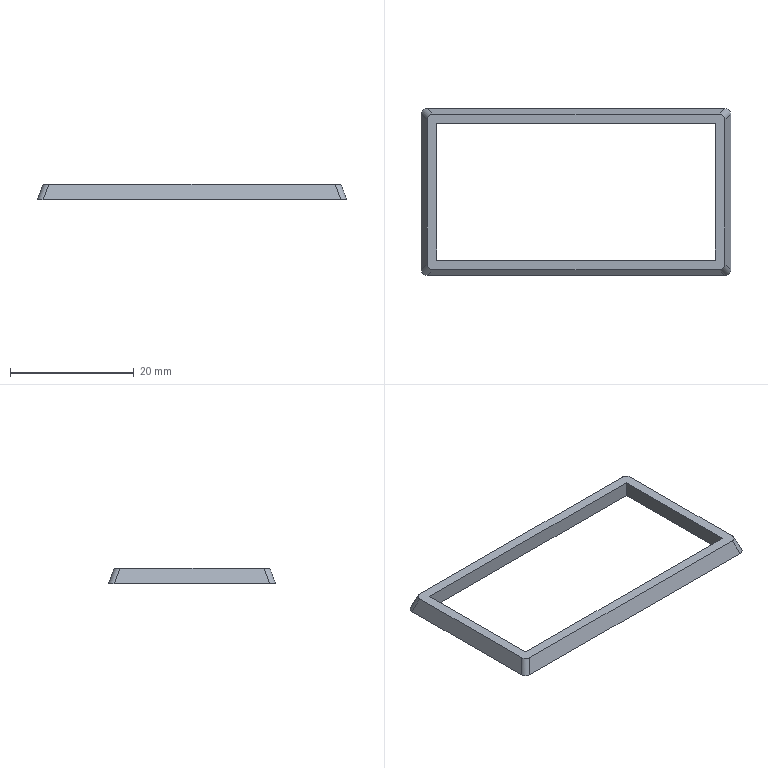Part | STEP file | Karet | 1 solid | 14 faces | box 50 x 27 x 2.5 mm | volume 725.773 mm3 | plane 10 | cylinder 4 | commonest cylinder face diameters 2 x4
STEP:
#1=CARTESIAN_POINT('',(0.,0.,0.));
#2=DIRECTION('',(0.,0.,1.));
#3=DIRECTION('',(1.,0.,0.));
#4=AXIS2_PLACEMENT_3D('',#1,#2,#3);
#5=CARTESIAN_POINT('',(24.09,-11.65,1.25));
#6=VERTEX_POINT('',#5);
#7=CARTESIAN_POINT('',(24.09,11.65,1.25));
#8=VERTEX_POINT('',#7);
#9=CARTESIAN_POINT('',(24.09,13.5,1.25));
#10=DIRECTION('',(0.,1.,0.));
#11=VECTOR('',#10,1.);
#12=LINE('',#9,#11);
#13=CARTESIAN_POINT('',(-25.,-13.5,1.25));
#14=DIRECTION('',(0.,0.,1.));
#15=DIRECTION('',(1.,0.,0.));
#16=AXIS2_PLACEMENT_3D('',#13,#14,#15);
#17=PLANE('',#16);
#18=CARTESIAN_POINT('',(49.09,27.));
#19=DIRECTION('',(0.,1.));
#20=VECTOR('',#19,1.);
#21=LINE('',#18,#20);
#22=(GEOMETRIC_REPRESENTATION_CONTEXT(2)PARAMETRIC_REPRESENTATION_CONTEXT()REPRESENTATION_CONTEXT('',''));
#23=DEFINITIONAL_REPRESENTATION('',(#21),#22);
#24=PCURVE('',#17,#23);
#25=CARTESIAN_POINT('',(24.09,-13.5,1.25));
#26=DIRECTION('',(0.9397,0.,0.342));
#27=DIRECTION('',(0.342,0.,-0.9397));
#28=AXIS2_PLACEMENT_3D('',#25,#26,#27);
#29=PLANE('',#28);
#30=CARTESIAN_POINT('',(0.,27.));
#31=DIRECTION('',(0.,1.));
#32=VECTOR('',#31,1.);
#33=LINE('',#30,#32);
#34=(GEOMETRIC_REPRESENTATION_CONTEXT(2)PARAMETRIC_REPRESENTATION_CONTEXT()REPRESENTATION_CONTEXT('',''));
#35=DEFINITIONAL_REPRESENTATION('',(#33),#34);
#36=PCURVE('',#29,#35);
#37=SURFACE_CURVE('',#12,(#24,#36),.PCURVE_S1.);
#38=EDGE_CURVE('',#6,#8,#37,.T.);
#39=ORIENTED_EDGE('',*,*,#38,.T.);
#40=CARTESIAN_POINT('',(23.15,12.59,1.25));
#41=VERTEX_POINT('',#40);
#42=CARTESIAN_POINT('',(24.09,11.65,1.25));
#43=CARTESIAN_POINT('',(24.09,12.213,1.25));
#44=CARTESIAN_POINT('',(23.713,12.59,1.25));
#45=CARTESIAN_POINT('',(23.15,12.59,1.25));
#46=(BOUNDED_CURVE()B_SPLINE_CURVE(3,(#42,#43,#44,#45),.UNSPECIFIED.,.F.,.F.)B_SPLINE_CURVE_WITH_KNOTS((4,4),(5.556,7.01),.PIECEWISE_BEZIER_KNOTS.)CURVE()GEOMETRIC_REPRESENTATION_ITEM()RATIONAL_B_SPLINE_CURVE((1.,0.8315,0.8315,1.))REPRESENTATION_ITEM(''));
#47=CARTESIAN_POINT('',(49.09,25.15));
#48=CARTESIAN_POINT('',(49.09,25.713));
#49=CARTESIAN_POINT('',(48.713,26.09));
#50=CARTESIAN_POINT('',(48.15,26.09));
#51=(BOUNDED_CURVE()B_SPLINE_CURVE(3,(#47,#48,#49,#50),.UNSPECIFIED.,.F.,.F.)B_SPLINE_CURVE_WITH_KNOTS((4,4),(5.556,7.01),.PIECEWISE_BEZIER_KNOTS.)CURVE()GEOMETRIC_REPRESENTATION_ITEM()RATIONAL_B_SPLINE_CURVE((1.,0.8315,0.8315,1.))REPRESENTATION_ITEM(''));
#52=(GEOMETRIC_REPRESENTATION_CONTEXT(2)PARAMETRIC_REPRESENTATION_CONTEXT()REPRESENTATION_CONTEXT('',''));
#53=DEFINITIONAL_REPRESENTATION('',(#51),#52);
#54=PCURVE('',#17,#53);
#55=CARTESIAN_POINT('',(18.108,6.608,14.763));
#56=DIRECTION('',(0.3236,0.3236,-0.8891));
#57=DIRECTION('',(-0.9397,0.,-0.342));
#58=AXIS2_PLACEMENT_3D('',#55,#56,#57);
#59=CYLINDRICAL_SURFACE('',#58,1.);
#60=CARTESIAN_POINT('',(3.142,15.582));
#61=CARTESIAN_POINT('',(3.121,15.589));
#62=CARTESIAN_POINT('',(3.081,15.603));
#63=CARTESIAN_POINT('',(3.018,15.622));
#64=CARTESIAN_POINT('',(2.955,15.639));
#65=CARTESIAN_POINT('',(2.89,15.656));
#66=CARTESIAN_POINT('',(2.824,15.67));
#67=CARTESIAN_POINT('',(2.757,15.683));
#68=CARTESIAN_POINT('',(2.69,15.693));
#69=CARTESIAN_POINT('',(2.622,15.702));
#70=CARTESIAN_POINT('',(2.553,15.708));
#71=CARTESIAN_POINT('',(2.484,15.711));
#72=CARTESIAN_POINT('',(2.415,15.713));
#73=CARTESIAN_POINT('',(2.346,15.711));
#74=CARTESIAN_POINT('',(2.277,15.708));
#75=CARTESIAN_POINT('',(2.208,15.702));
#76=CARTESIAN_POINT('',(2.14,15.693));
#77=CARTESIAN_POINT('',(2.072,15.683));
#78=CARTESIAN_POINT('',(2.006,15.67));
#79=CARTESIAN_POINT('',(1.94,15.656));
#80=CARTESIAN_POINT('',(1.875,15.639));
#81=CARTESIAN_POINT('',(1.811,15.622));
#82=CARTESIAN_POINT('',(1.749,15.603));
#83=CARTESIAN_POINT('',(1.708,15.589));
#84=CARTESIAN_POINT('',(1.688,15.582));
#85=B_SPLINE_CURVE_WITH_KNOTS('',3,(#60,#61,#62,#63,#64,#65,#66,#67,#68,#69,#70,#71,#72,#73,#74,#75,#76,#77,#78,#79,#80,#81,#82,#83,#84),.UNSPECIFIED.,.F.,.F.,(4,1,1,1,1,1,1,1,1,1,1,1,1,1,1,1,1,1,1,1,1,1,4),(5.556,5.622,5.689,5.755,5.821,5.887,5.953,6.019,6.085,6.151,6.217,6.283,6.349,6.415,6.481,6.547,6.614,6.68,6.746,6.812,6.878,6.944,7.01),.QUASI_UNIFORM_KNOTS.);
#86=(GEOMETRIC_REPRESENTATION_CONTEXT(2)PARAMETRIC_REPRESENTATION_CONTEXT()REPRESENTATION_CONTEXT('',''));
#87=DEFINITIONAL_REPRESENTATION('',(#85),#86);
#88=PCURVE('',#59,#87);
#89=SURFACE_CURVE('',#46,(#54,#88),.PCURVE_S1.);
#90=EDGE_CURVE('',#8,#41,#89,.T.);
#91=ORIENTED_EDGE('',*,*,#90,.T.);
#92=CARTESIAN_POINT('',(-23.15,12.59,1.25));
#93=VERTEX_POINT('',#92);
#94=CARTESIAN_POINT('',(-25.,12.59,1.25));
#95=DIRECTION('',(-1.,0.,0.));
#96=VECTOR('',#95,1.);
#97=LINE('',#94,#96);
#98=CARTESIAN_POINT('',(0.,26.09));
#99=DIRECTION('',(-1.,0.));
#100=VECTOR('',#99,1.);
#101=LINE('',#98,#100);
#102=(GEOMETRIC_REPRESENTATION_CONTEXT(2)PARAMETRIC_REPRESENTATION_CONTEXT()REPRESENTATION_CONTEXT('',''));
#103=DEFINITIONAL_REPRESENTATION('',(#101),#102);
#104=PCURVE('',#17,#103);
#105=CARTESIAN_POINT('',(-25.,12.59,1.25));
#106=DIRECTION('',(0.,0.9397,0.342));
#107=DIRECTION('',(0.,-0.342,0.9397));
#108=AXIS2_PLACEMENT_3D('',#105,#106,#107);
#109=PLANE('',#108);
#110=CARTESIAN_POINT('',(0.,0.));
#111=DIRECTION('',(0.,-1.));
#112=VECTOR('',#111,1.);
#113=LINE('',#110,#112);
#114=(GEOMETRIC_REPRESENTATION_CONTEXT(2)PARAMETRIC_REPRESENTATION_CONTEXT()REPRESENTATION_CONTEXT('',''));
#115=DEFINITIONAL_REPRESENTATION('',(#113),#114);
#116=PCURVE('',#109,#115);
#117=SURFACE_CURVE('',#97,(#104,#116),.PCURVE_S1.);
#118=EDGE_CURVE('',#41,#93,#117,.T.);
#119=ORIENTED_EDGE('',*,*,#118,.T.);
#120=CARTESIAN_POINT('',(-24.09,11.65,1.25));
#121=VERTEX_POINT('',#120);
#122=CARTESIAN_POINT('',(-23.15,12.59,1.25));
#123=CARTESIAN_POINT('',(-23.713,12.59,1.25));
#124=CARTESIAN_POINT('',(-24.09,12.213,1.25));
#125=CARTESIAN_POINT('',(-24.09,11.65,1.25));
#126=(BOUNDED_CURVE()B_SPLINE_CURVE(3,(#122,#123,#124,#125),.UNSPECIFIED.,.F.,.F.)B_SPLINE_CURVE_WITH_KNOTS((4,4),(5.556,7.01),.PIECEWISE_BEZIER_KNOTS.)CURVE()GEOMETRIC_REPRESENTATION_ITEM()RATIONAL_B_SPLINE_CURVE((1.,0.8315,0.8315,1.))REPRESENTATION_ITEM(''));
#127=CARTESIAN_POINT('',(1.85,26.09));
#128=CARTESIAN_POINT('',(1.287,26.09));
#129=CARTESIAN_POINT('',(0.9099,25.713));
#130=CARTESIAN_POINT('',(0.9099,25.15));
#131=(BOUNDED_CURVE()B_SPLINE_CURVE(3,(#127,#128,#129,#130),.UNSPECIFIED.,.F.,.F.)B_SPLINE_CURVE_WITH_KNOTS((4,4),(5.556,7.01),.PIECEWISE_BEZIER_KNOTS.)CURVE()GEOMETRIC_REPRESENTATION_ITEM()RATIONAL_B_SPLINE_CURVE((1.,0.8315,0.8315,1.))REPRESENTATION_ITEM(''));
#132=(GEOMETRIC_REPRESENTATION_CONTEXT(2)PARAMETRIC_REPRESENTATION_CONTEXT()REPRESENTATION_CONTEXT('',''));
#133=DEFINITIONAL_REPRESENTATION('',(#131),#132);
#134=PCURVE('',#17,#133);
#135=CARTESIAN_POINT('',(-20.516,9.016,8.145));
#136=DIRECTION('',(-0.3236,0.3236,-0.8891));
#137=DIRECTION('',(-0.9397,0.,0.342));
#138=AXIS2_PLACEMENT_3D('',#135,#136,#137);
#139=CYLINDRICAL_SURFACE('',#138,1.);
#140=CARTESIAN_POINT('',(1.454,8.139));
#141=CARTESIAN_POINT('',(1.433,8.146));
#142=CARTESIAN_POINT('',(1.393,8.159));
#143=CARTESIAN_POINT('',(1.33,8.178));
#144=CARTESIAN_POINT('',(1.267,8.196));
#145=CARTESIAN_POINT('',(1.202,8.212));
#146=CARTESIAN_POINT('',(1.136,8.227));
#147=CARTESIAN_POINT('',(1.069,8.24));
#148=CARTESIAN_POINT('',(1.002,8.25));
#149=CARTESIAN_POINT('',(0.9335,8.259));
#150=CARTESIAN_POINT('',(0.8649,8.265));
#151=CARTESIAN_POINT('',(0.7959,8.268));
#152=CARTESIAN_POINT('',(0.7268,8.27));
#153=CARTESIAN_POINT('',(0.6576,8.268));
#154=CARTESIAN_POINT('',(0.5887,8.265));
#155=CARTESIAN_POINT('',(0.52,8.259));
#156=CARTESIAN_POINT('',(0.4518,8.25));
#157=CARTESIAN_POINT('',(0.3843,8.24));
#158=CARTESIAN_POINT('',(0.3176,8.227));
#159=CARTESIAN_POINT('',(0.2517,8.212));
#160=CARTESIAN_POINT('',(0.1869,8.196));
#161=CARTESIAN_POINT('',(0.1233,8.178));
#162=CARTESIAN_POINT('',(0.06087,8.159));
#163=CARTESIAN_POINT('',(0.02013,8.146));
#164=CARTESIAN_POINT('',(0.,8.139));
#165=B_SPLINE_CURVE_WITH_KNOTS('',3,(#140,#141,#142,#143,#144,#145,#146,#147,#148,#149,#150,#151,#152,#153,#154,#155,#156,#157,#158,#159,#160,#161,#162,#163,#164),.UNSPECIFIED.,.F.,.F.,(4,1,1,1,1,1,1,1,1,1,1,1,1,1,1,1,1,1,1,1,1,1,4),(5.556,5.622,5.689,5.755,5.821,5.887,5.953,6.019,6.085,6.151,6.217,6.283,6.349,6.415,6.481,6.547,6.614,6.68,6.746,6.812,6.878,6.944,7.01),.QUASI_UNIFORM_KNOTS.);
#166=(GEOMETRIC_REPRESENTATION_CONTEXT(2)PARAMETRIC_REPRESENTATION_CONTEXT()REPRESENTATION_CONTEXT('',''));
#167=DEFINITIONAL_REPRESENTATION('',(#165),#166);
#168=PCURVE('',#139,#167);
#169=SURFACE_CURVE('',#126,(#134,#168),.PCURVE_S1.);
#170=EDGE_CURVE('',#93,#121,#169,.T.);
#171=ORIENTED_EDGE('',*,*,#170,.T.);
#172=CARTESIAN_POINT('',(-24.09,-11.65,1.25));
#173=VERTEX_POINT('',#172);
#174=CARTESIAN_POINT('',(-24.09,-13.5,1.25));
#175=DIRECTION('',(0.,-1.,0.));
#176=VECTOR('',#175,1.);
#177=LINE('',#174,#176);
#178=CARTESIAN_POINT('',(0.9099,0.));
#179=DIRECTION('',(0.,-1.));
#180=VECTOR('',#179,1.);
#181=LINE('',#178,#180);
#182=(GEOMETRIC_REPRESENTATION_CONTEXT(2)PARAMETRIC_REPRESENTATION_CONTEXT()REPRESENTATION_CONTEXT('',''));
#183=DEFINITIONAL_REPRESENTATION('',(#181),#182);
#184=PCURVE('',#17,#183);
#185=CARTESIAN_POINT('',(-24.09,-13.5,1.25));
#186=DIRECTION('',(-0.9397,0.,0.342));
#187=DIRECTION('',(0.342,0.,0.9397));
#188=AXIS2_PLACEMENT_3D('',#185,#186,#187);
#189=PLANE('',#188);
#190=CARTESIAN_POINT('',(0.,0.));
#191=DIRECTION('',(0.,-1.));
#192=VECTOR('',#191,1.);
#193=LINE('',#190,#192);
#194=(GEOMETRIC_REPRESENTATION_CONTEXT(2)PARAMETRIC_REPRESENTATION_CONTEXT()REPRESENTATION_CONTEXT('',''));
#195=DEFINITIONAL_REPRESENTATION('',(#193),#194);
#196=PCURVE('',#189,#195);
#197=SURFACE_CURVE('',#177,(#184,#196),.PCURVE_S1.);
#198=EDGE_CURVE('',#121,#173,#197,.T.);
#199=ORIENTED_EDGE('',*,*,#198,.T.);
#200=CARTESIAN_POINT('',(-23.15,-12.59,1.25));
#201=VERTEX_POINT('',#200);
#202=CARTESIAN_POINT('',(-24.09,-11.65,1.25));
#203=CARTESIAN_POINT('',(-24.09,-12.213,1.25));
#204=CARTESIAN_POINT('',(-23.713,-12.59,1.25));
#205=CARTESIAN_POINT('',(-23.15,-12.59,1.25));
#206=(BOUNDED_CURVE()B_SPLINE_CURVE(3,(#202,#203,#204,#205),.UNSPECIFIED.,.F.,.F.)B_SPLINE_CURVE_WITH_KNOTS((4,4),(2.415,3.868),.PIECEWISE_BEZIER_KNOTS.)CURVE()GEOMETRIC_REPRESENTATION_ITEM()RATIONAL_B_SPLINE_CURVE((1.,0.8315,0.8315,1.))REPRESENTATION_ITEM(''));
#207=CARTESIAN_POINT('',(0.9099,1.85));
#208=CARTESIAN_POINT('',(0.9099,1.287));
#209=CARTESIAN_POINT('',(1.287,0.9099));
#210=CARTESIAN_POINT('',(1.85,0.9099));
#211=(BOUNDED_CURVE()B_SPLINE_CURVE(3,(#207,#208,#209,#210),.UNSPECIFIED.,.F.,.F.)B_SPLINE_CURVE_WITH_KNOTS((4,4),(2.415,3.868),.PIECEWISE_BEZIER_KNOTS.)CURVE()GEOMETRIC_REPRESENTATION_ITEM()RATIONAL_B_SPLINE_CURVE((1.,0.8315,0.8315,1.))REPRESENTATION_ITEM(''));
#212=(GEOMETRIC_REPRESENTATION_CONTEXT(2)PARAMETRIC_REPRESENTATION_CONTEXT()REPRESENTATION_CONTEXT('',''));
#213=DEFINITIONAL_REPRESENTATION('',(#211),#212);
#214=PCURVE('',#17,#213);
#215=CARTESIAN_POINT('',(-23.344,-11.844,0.3758));
#216=DIRECTION('',(0.3236,0.3236,0.8891));
#217=DIRECTION('',(0.9397,0.,-0.342));
#218=AXIS2_PLACEMENT_3D('',#215,#216,#217);
#219=CYLINDRICAL_SURFACE('',#218,1.);
#220=CARTESIAN_POINT('',(3.142,0.5986));
#221=CARTESIAN_POINT('',(3.162,0.5917));
#222=CARTESIAN_POINT('',(3.202,0.5782));
#223=CARTESIAN_POINT('',(3.265,0.5591));
#224=CARTESIAN_POINT('',(3.329,0.5414));
#225=CARTESIAN_POINT('',(3.393,0.5252));
#226=CARTESIAN_POINT('',(3.459,0.5107));
#227=CARTESIAN_POINT('',(3.526,0.498));
#228=CARTESIAN_POINT('',(3.593,0.4875));
#229=CARTESIAN_POINT('',(3.662,0.4791));
#230=CARTESIAN_POINT('',(3.73,0.473));
#231=CARTESIAN_POINT('',(3.799,0.4693));
#232=CARTESIAN_POINT('',(3.868,0.4681));
#233=CARTESIAN_POINT('',(3.938,0.4693));
#234=CARTESIAN_POINT('',(4.006,0.473));
#235=CARTESIAN_POINT('',(4.075,0.4791));
#236=CARTESIAN_POINT('',(4.143,0.4875));
#237=CARTESIAN_POINT('',(4.211,0.498));
#238=CARTESIAN_POINT('',(4.278,0.5107));
#239=CARTESIAN_POINT('',(4.343,0.5252));
#240=CARTESIAN_POINT('',(4.408,0.5414));
#241=CARTESIAN_POINT('',(4.472,0.5591));
#242=CARTESIAN_POINT('',(4.534,0.5782));
#243=CARTESIAN_POINT('',(4.575,0.5917));
#244=CARTESIAN_POINT('',(4.595,0.5986));
#245=B_SPLINE_CURVE_WITH_KNOTS('',3,(#220,#221,#222,#223,#224,#225,#226,#227,#228,#229,#230,#231,#232,#233,#234,#235,#236,#237,#238,#239,#240,#241,#242,#243,#244),.UNSPECIFIED.,.F.,.F.,(4,1,1,1,1,1,1,1,1,1,1,1,1,1,1,1,1,1,1,1,1,1,4),(2.415,2.481,2.547,2.613,2.679,2.745,2.811,2.877,2.943,3.009,3.076,3.142,3.208,3.274,3.34,3.406,3.472,3.538,3.604,3.67,3.736,3.802,3.868),.QUASI_UNIFORM_KNOTS.);
#246=(GEOMETRIC_REPRESENTATION_CONTEXT(2)PARAMETRIC_REPRESENTATION_CONTEXT()REPRESENTATION_CONTEXT('',''));
#247=DEFINITIONAL_REPRESENTATION('',(#245),#246);
#248=PCURVE('',#219,#247);
#249=SURFACE_CURVE('',#206,(#214,#248),.PCURVE_S1.);
#250=EDGE_CURVE('',#173,#201,#249,.T.);
#251=ORIENTED_EDGE('',*,*,#250,.T.);
#252=CARTESIAN_POINT('',(23.15,-12.59,1.25));
#253=VERTEX_POINT('',#252);
#254=CARTESIAN_POINT('',(25.,-12.59,1.25));
#255=DIRECTION('',(1.,0.,0.));
#256=VECTOR('',#255,1.);
#257=LINE('',#254,#256);
#258=CARTESIAN_POINT('',(50.,0.9099));
#259=DIRECTION('',(1.,0.));
#260=VECTOR('',#259,1.);
#261=LINE('',#258,#260);
#262=(GEOMETRIC_REPRESENTATION_CONTEXT(2)PARAMETRIC_REPRESENTATION_CONTEXT()REPRESENTATION_CONTEXT('',''));
#263=DEFINITIONAL_REPRESENTATION('',(#261),#262);
#264=PCURVE('',#17,#263);
#265=CARTESIAN_POINT('',(-25.,-12.59,1.25));
#266=DIRECTION('',(0.,-0.9397,0.342));
#267=DIRECTION('',(0.,-0.342,-0.9397));
#268=AXIS2_PLACEMENT_3D('',#265,#266,#267);
#269=PLANE('',#268);
#270=CARTESIAN_POINT('',(0.,50.));
#271=DIRECTION('',(0.,1.));
#272=VECTOR('',#271,1.);
#273=LINE('',#270,#272);
#274=(GEOMETRIC_REPRESENTATION_CONTEXT(2)PARAMETRIC_REPRESENTATION_CONTEXT()REPRESENTATION_CONTEXT('',''));
#275=DEFINITIONAL_REPRESENTATION('',(#273),#274);
#276=PCURVE('',#269,#275);
#277=SURFACE_CURVE('',#257,(#264,#276),.PCURVE_S1.);
#278=EDGE_CURVE('',#201,#253,#277,.T.);
#279=ORIENTED_EDGE('',*,*,#278,.T.);
#280=CARTESIAN_POINT('',(23.15,-12.59,1.25));
#281=CARTESIAN_POINT('',(23.713,-12.59,1.25));
#282=CARTESIAN_POINT('',(24.09,-12.213,1.25));
#283=CARTESIAN_POINT('',(24.09,-11.65,1.25));
#284=(BOUNDED_CURVE()B_SPLINE_CURVE(3,(#280,#281,#282,#283),.UNSPECIFIED.,.F.,.F.)B_SPLINE_CURVE_WITH_KNOTS((4,4),(2.415,3.868),.PIECEWISE_BEZIER_KNOTS.)CURVE()GEOMETRIC_REPRESENTATION_ITEM()RATIONAL_B_SPLINE_CURVE((1.,0.8315,0.8315,1.))REPRESENTATION_ITEM(''));
#285=CARTESIAN_POINT('',(48.15,0.9099));
#286=CARTESIAN_POINT('',(48.713,0.9099));
#287=CARTESIAN_POINT('',(49.09,1.287));
#288=CARTESIAN_POINT('',(49.09,1.85));
#289=(BOUNDED_CURVE()B_SPLINE_CURVE(3,(#285,#286,#287,#288),.UNSPECIFIED.,.F.,.F.)B_SPLINE_CURVE_WITH_KNOTS((4,4),(2.415,3.868),.PIECEWISE_BEZIER_KNOTS.)CURVE()GEOMETRIC_REPRESENTATION_ITEM()RATIONAL_B_SPLINE_CURVE((1.,0.8315,0.8315,1.))REPRESENTATION_ITEM(''));
#290=(GEOMETRIC_REPRESENTATION_CONTEXT(2)PARAMETRIC_REPRESENTATION_CONTEXT()REPRESENTATION_CONTEXT('',''));
#291=DEFINITIONAL_REPRESENTATION('',(#289),#290);
#292=PCURVE('',#17,#291);
#293=CARTESIAN_POINT('',(18.108,-6.608,14.763));
#294=DIRECTION('',(-0.3236,0.3236,0.8891));
#295=DIRECTION('',(0.9397,0.,0.342));
#296=AXIS2_PLACEMENT_3D('',#293,#294,#295);
#297=CYLINDRICAL_SURFACE('',#296,1.);
#298=CARTESIAN_POINT('',(4.83,-15.582));
#299=CARTESIAN_POINT('',(4.85,-15.589));
#300=CARTESIAN_POINT('',(4.891,-15.603));
#301=CARTESIAN_POINT('',(4.953,-15.622));
#302=CARTESIAN_POINT('',(5.017,-15.639));
#303=CARTESIAN_POINT('',(5.081,-15.656));
#304=CARTESIAN_POINT('',(5.147,-15.67));
#305=CARTESIAN_POINT('',(5.214,-15.683));
#306=CARTESIAN_POINT('',(5.281,-15.693));
#307=CARTESIAN_POINT('',(5.35,-15.702));
#308=CARTESIAN_POINT('',(5.418,-15.708));
#309=CARTESIAN_POINT('',(5.487,-15.711));
#310=CARTESIAN_POINT('',(5.556,-15.713));
#311=CARTESIAN_POINT('',(5.626,-15.711));
#312=CARTESIAN_POINT('',(5.695,-15.708));
#313=CARTESIAN_POINT('',(5.763,-15.702));
#314=CARTESIAN_POINT('',(5.831,-15.693));
#315=CARTESIAN_POINT('',(5.899,-15.683));
#316=CARTESIAN_POINT('',(5.966,-15.67));
#317=CARTESIAN_POINT('',(6.031,-15.656));
#318=CARTESIAN_POINT('',(6.096,-15.639));
#319=CARTESIAN_POINT('',(6.16,-15.622));
#320=CARTESIAN_POINT('',(6.222,-15.603));
#321=CARTESIAN_POINT('',(6.263,-15.589));
#322=CARTESIAN_POINT('',(6.283,-15.582));
#323=B_SPLINE_CURVE_WITH_KNOTS('',3,(#298,#299,#300,#301,#302,#303,#304,#305,#306,#307,#308,#309,#310,#311,#312,#313,#314,#315,#316,#317,#318,#319,#320,#321,#322),.UNSPECIFIED.,.F.,.F.,(4,1,1,1,1,1,1,1,1,1,1,1,1,1,1,1,1,1,1,1,1,1,4),(2.415,2.481,2.547,2.613,2.679,2.745,2.811,2.877,2.943,3.009,3.076,3.142,3.208,3.274,3.34,3.406,3.472,3.538,3.604,3.67,3.736,3.802,3.868),.QUASI_UNIFORM_KNOTS.);
#324=(GEOMETRIC_REPRESENTATION_CONTEXT(2)PARAMETRIC_REPRESENTATION_CONTEXT()REPRESENTATION_CONTEXT('',''));
#325=DEFINITIONAL_REPRESENTATION('',(#323),#324);
#326=PCURVE('',#297,#325);
#327=SURFACE_CURVE('',#284,(#292,#326),.PCURVE_S1.);
#328=EDGE_CURVE('',#253,#6,#327,.T.);
#329=ORIENTED_EDGE('',*,*,#328,.T.);
#330=EDGE_LOOP('',(#39,#91,#119,#171,#199,#251,#279,#329));
#331=FACE_BOUND('',#330,.T.);
#332=CARTESIAN_POINT('',(22.5,11.,1.25));
#333=VERTEX_POINT('',#332);
#334=CARTESIAN_POINT('',(-22.5,11.,1.25));
#335=VERTEX_POINT('',#334);
#336=CARTESIAN_POINT('',(-22.5,11.,1.25));
#337=DIRECTION('',(-1.,0.,0.));
#338=VECTOR('',#337,1.);
#339=LINE('',#336,#338);
#340=CARTESIAN_POINT('',(2.5,24.5));
#341=DIRECTION('',(-1.,0.));
#342=VECTOR('',#341,1.);
#343=LINE('',#340,#342);
#344=(GEOMETRIC_REPRESENTATION_CONTEXT(2)PARAMETRIC_REPRESENTATION_CONTEXT()REPRESENTATION_CONTEXT('',''));
#345=DEFINITIONAL_REPRESENTATION('',(#343),#344);
#346=PCURVE('',#17,#345);
#347=CARTESIAN_POINT('',(-22.5,11.,1.25));
#348=DIRECTION('',(0.,-1.,0.));
#349=DIRECTION('',(0.,0.,-1.));
#350=AXIS2_PLACEMENT_3D('',#347,#348,#349);
#351=PLANE('',#350);
#352=CARTESIAN_POINT('',(0.,0.));
#353=DIRECTION('',(0.,-1.));
#354=VECTOR('',#353,1.);
#355=LINE('',#352,#354);
#356=(GEOMETRIC_REPRESENTATION_CONTEXT(2)PARAMETRIC_REPRESENTATION_CONTEXT()REPRESENTATION_CONTEXT('',''));
#357=DEFINITIONAL_REPRESENTATION('',(#355),#356);
#358=PCURVE('',#351,#357);
#359=SURFACE_CURVE('',#339,(#346,#358),.PCURVE_S1.);
#360=EDGE_CURVE('',#333,#335,#359,.T.);
#361=ORIENTED_EDGE('',*,*,#360,.F.);
#362=CARTESIAN_POINT('',(22.5,-11.,1.25));
#363=VERTEX_POINT('',#362);
#364=CARTESIAN_POINT('',(22.5,11.,1.25));
#365=DIRECTION('',(0.,1.,0.));
#366=VECTOR('',#365,1.);
#367=LINE('',#364,#366);
#368=CARTESIAN_POINT('',(47.5,24.5));
#369=DIRECTION('',(0.,1.));
#370=VECTOR('',#369,1.);
#371=LINE('',#368,#370);
#372=(GEOMETRIC_REPRESENTATION_CONTEXT(2)PARAMETRIC_REPRESENTATION_CONTEXT()REPRESENTATION_CONTEXT('',''));
#373=DEFINITIONAL_REPRESENTATION('',(#371),#372);
#374=PCURVE('',#17,#373);
#375=CARTESIAN_POINT('',(22.5,11.,1.25));
#376=DIRECTION('',(-1.,0.,0.));
#377=DIRECTION('',(0.,-1.,0.));
#378=AXIS2_PLACEMENT_3D('',#375,#376,#377);
#379=PLANE('',#378);
#380=CARTESIAN_POINT('',(0.,0.));
#381=DIRECTION('',(-1.,0.));
#382=VECTOR('',#381,1.);
#383=LINE('',#380,#382);
#384=(GEOMETRIC_REPRESENTATION_CONTEXT(2)PARAMETRIC_REPRESENTATION_CONTEXT()REPRESENTATION_CONTEXT('',''));
#385=DEFINITIONAL_REPRESENTATION('',(#383),#384);
#386=PCURVE('',#379,#385);
#387=SURFACE_CURVE('',#367,(#374,#386),.PCURVE_S1.);
#388=EDGE_CURVE('',#363,#333,#387,.T.);
#389=ORIENTED_EDGE('',*,*,#388,.F.);
#390=CARTESIAN_POINT('',(-22.5,-11.,1.25));
#391=VERTEX_POINT('',#390);
#392=CARTESIAN_POINT('',(-22.5,-11.,1.25));
#393=DIRECTION('',(1.,0.,0.));
#394=VECTOR('',#393,1.);
#395=LINE('',#392,#394);
#396=CARTESIAN_POINT('',(2.5,2.5));
#397=DIRECTION('',(1.,0.));
#398=VECTOR('',#397,1.);
#399=LINE('',#396,#398);
#400=(GEOMETRIC_REPRESENTATION_CONTEXT(2)PARAMETRIC_REPRESENTATION_CONTEXT()REPRESENTATION_CONTEXT('',''));
#401=DEFINITIONAL_REPRESENTATION('',(#399),#400);
#402=PCURVE('',#17,#401);
#403=CARTESIAN_POINT('',(-22.5,-11.,1.25));
#404=DIRECTION('',(0.,1.,0.));
#405=DIRECTION('',(0.,0.,1.));
#406=AXIS2_PLACEMENT_3D('',#403,#404,#405);
#407=PLANE('',#406);
#408=CARTESIAN_POINT('',(0.,0.));
#409=DIRECTION('',(0.,1.));
#410=VECTOR('',#409,1.);
#411=LINE('',#408,#410);
#412=(GEOMETRIC_REPRESENTATION_CONTEXT(2)PARAMETRIC_REPRESENTATION_CONTEXT()REPRESENTATION_CONTEXT('',''));
#413=DEFINITIONAL_REPRESENTATION('',(#411),#412);
#414=PCURVE('',#407,#413);
#415=SURFACE_CURVE('',#395,(#402,#414),.PCURVE_S1.);
#416=EDGE_CURVE('',#391,#363,#415,.T.);
#417=ORIENTED_EDGE('',*,*,#416,.F.);
#418=CARTESIAN_POINT('',(-22.5,11.,1.25));
#419=DIRECTION('',(0.,-1.,0.));
#420=VECTOR('',#419,1.);
#421=LINE('',#418,#420);
#422=CARTESIAN_POINT('',(2.5,24.5));
#423=DIRECTION('',(0.,-1.));
#424=VECTOR('',#423,1.);
#425=LINE('',#422,#424);
#426=(GEOMETRIC_REPRESENTATION_CONTEXT(2)PARAMETRIC_REPRESENTATION_CONTEXT()REPRESENTATION_CONTEXT('',''));
#427=DEFINITIONAL_REPRESENTATION('',(#425),#426);
#428=PCURVE('',#17,#427);
#429=CARTESIAN_POINT('',(-22.5,11.,1.25));
#430=DIRECTION('',(1.,0.,0.));
#431=DIRECTION('',(0.,1.,0.));
#432=AXIS2_PLACEMENT_3D('',#429,#430,#431);
#433=PLANE('',#432);
#434=CARTESIAN_POINT('',(0.,0.));
#435=DIRECTION('',(-1.,0.));
#436=VECTOR('',#435,1.);
#437=LINE('',#434,#436);
#438=(GEOMETRIC_REPRESENTATION_CONTEXT(2)PARAMETRIC_REPRESENTATION_CONTEXT()REPRESENTATION_CONTEXT('',''));
#439=DEFINITIONAL_REPRESENTATION('',(#437),#438);
#440=PCURVE('',#433,#439);
#441=SURFACE_CURVE('',#421,(#428,#440),.PCURVE_S1.);
#442=EDGE_CURVE('',#335,#391,#441,.T.);
#443=ORIENTED_EDGE('',*,*,#442,.F.);
#444=EDGE_LOOP('',(#361,#389,#417,#443));
#445=FACE_BOUND('',#444,.T.);
#446=ADVANCED_FACE('',(#331,#445),#17,.T.);
#447=CARTESIAN_POINT('',(24.06,13.5,-1.25));
#448=VERTEX_POINT('',#447);
#449=CARTESIAN_POINT('',(-24.06,13.5,-1.25));
#450=VERTEX_POINT('',#449);
#451=CARTESIAN_POINT('',(-25.,13.5,-1.25));
#452=DIRECTION('',(-1.,0.,0.));
#453=VECTOR('',#452,1.);
#454=LINE('',#451,#453);
#455=CARTESIAN_POINT('',(-25.,-13.5,-1.25));
#456=DIRECTION('',(0.,0.,1.));
#457=DIRECTION('',(1.,0.,0.));
#458=AXIS2_PLACEMENT_3D('',#455,#456,#457);
#459=PLANE('',#458);
#460=CARTESIAN_POINT('',(0.,27.));
#461=DIRECTION('',(-1.,0.));
#462=VECTOR('',#461,1.);
#463=LINE('',#460,#462);
#464=(GEOMETRIC_REPRESENTATION_CONTEXT(2)PARAMETRIC_REPRESENTATION_CONTEXT()REPRESENTATION_CONTEXT('',''));
#465=DEFINITIONAL_REPRESENTATION('',(#463),#464);
#466=PCURVE('',#459,#465);
#467=CARTESIAN_POINT('',(-2.66,0.));
#468=DIRECTION('',(0.,-1.));
#469=VECTOR('',#468,1.);
#470=LINE('',#467,#469);
#471=(GEOMETRIC_REPRESENTATION_CONTEXT(2)PARAMETRIC_REPRESENTATION_CONTEXT()REPRESENTATION_CONTEXT('',''));
#472=DEFINITIONAL_REPRESENTATION('',(#470),#471);
#473=PCURVE('',#109,#472);
#474=SURFACE_CURVE('',#454,(#466,#473),.PCURVE_S1.);
#475=EDGE_CURVE('',#448,#450,#474,.T.);
#476=ORIENTED_EDGE('',*,*,#475,.F.);
#477=CARTESIAN_POINT('',(25.,12.56,-1.25));
#478=VERTEX_POINT('',#477);
#479=CARTESIAN_POINT('',(24.06,13.5,-1.25));
#480=CARTESIAN_POINT('',(24.623,13.5,-1.25));
#481=CARTESIAN_POINT('',(25.,13.123,-1.25));
#482=CARTESIAN_POINT('',(25.,12.56,-1.25));
#483=(BOUNDED_CURVE()B_SPLINE_CURVE(3,(#479,#480,#481,#482),.UNSPECIFIED.,.F.,.F.)B_SPLINE_CURVE_WITH_KNOTS((4,4),(5.556,7.01),.PIECEWISE_BEZIER_KNOTS.)CURVE()GEOMETRIC_REPRESENTATION_ITEM()RATIONAL_B_SPLINE_CURVE((1.,0.8315,0.8315,1.))REPRESENTATION_ITEM(''));
#484=CARTESIAN_POINT('',(49.06,27.));
#485=CARTESIAN_POINT('',(49.623,27.));
#486=CARTESIAN_POINT('',(50.,26.623));
#487=CARTESIAN_POINT('',(50.,26.06));
#488=(BOUNDED_CURVE()B_SPLINE_CURVE(3,(#484,#485,#486,#487),.UNSPECIFIED.,.F.,.F.)B_SPLINE_CURVE_WITH_KNOTS((4,4),(5.556,7.01),.PIECEWISE_BEZIER_KNOTS.)CURVE()GEOMETRIC_REPRESENTATION_ITEM()RATIONAL_B_SPLINE_CURVE((1.,0.8315,0.8315,1.))REPRESENTATION_ITEM(''));
#489=(GEOMETRIC_REPRESENTATION_CONTEXT(2)PARAMETRIC_REPRESENTATION_CONTEXT()REPRESENTATION_CONTEXT('',''));
#490=DEFINITIONAL_REPRESENTATION('',(#488),#489);
#491=PCURVE('',#459,#490);
#492=CARTESIAN_POINT('',(1.688,18.394));
#493=CARTESIAN_POINT('',(1.708,18.401));
#494=CARTESIAN_POINT('',(1.749,18.414));
#495=CARTESIAN_POINT('',(1.811,18.433));
#496=CARTESIAN_POINT('',(1.875,18.451));
#497=CARTESIAN_POINT('',(1.94,18.467));
#498=CARTESIAN_POINT('',(2.006,18.482));
#499=CARTESIAN_POINT('',(2.072,18.494));
#500=CARTESIAN_POINT('',(2.14,18.505));
#501=CARTESIAN_POINT('',(2.208,18.513));
#502=CARTESIAN_POINT('',(2.277,18.52));
#503=CARTESIAN_POINT('',(2.346,18.523));
#504=CARTESIAN_POINT('',(2.415,18.524));
#505=CARTESIAN_POINT('',(2.484,18.523));
#506=CARTESIAN_POINT('',(2.553,18.52));
#507=CARTESIAN_POINT('',(2.622,18.513));
#508=CARTESIAN_POINT('',(2.69,18.505));
#509=CARTESIAN_POINT('',(2.757,18.494));
#510=CARTESIAN_POINT('',(2.824,18.482));
#511=CARTESIAN_POINT('',(2.89,18.467));
#512=CARTESIAN_POINT('',(2.955,18.451));
#513=CARTESIAN_POINT('',(3.018,18.433));
#514=CARTESIAN_POINT('',(3.081,18.414));
#515=CARTESIAN_POINT('',(3.121,18.401));
#516=CARTESIAN_POINT('',(3.142,18.394));
#517=B_SPLINE_CURVE_WITH_KNOTS('',3,(#492,#493,#494,#495,#496,#497,#498,#499,#500,#501,#502,#503,#504,#505,#506,#507,#508,#509,#510,#511,#512,#513,#514,#515,#516),.UNSPECIFIED.,.F.,.F.,(4,1,1,1,1,1,1,1,1,1,1,1,1,1,1,1,1,1,1,1,1,1,4),(5.556,5.622,5.689,5.755,5.821,5.887,5.953,6.019,6.085,6.151,6.217,6.283,6.349,6.415,6.481,6.547,6.614,6.68,6.746,6.812,6.878,6.944,7.01),.QUASI_UNIFORM_KNOTS.);
#518=(GEOMETRIC_REPRESENTATION_CONTEXT(2)PARAMETRIC_REPRESENTATION_CONTEXT()REPRESENTATION_CONTEXT('',''));
#519=DEFINITIONAL_REPRESENTATION('',(#517),#518);
#520=PCURVE('',#59,#519);
#521=SURFACE_CURVE('',#483,(#491,#520),.PCURVE_S1.);
#522=EDGE_CURVE('',#448,#478,#521,.T.);
#523=ORIENTED_EDGE('',*,*,#522,.T.);
#524=CARTESIAN_POINT('',(25.,-12.56,-1.25));
#525=VERTEX_POINT('',#524);
#526=CARTESIAN_POINT('',(25.,13.5,-1.25));
#527=DIRECTION('',(0.,1.,0.));
#528=VECTOR('',#527,1.);
#529=LINE('',#526,#528);
#530=CARTESIAN_POINT('',(50.,27.));
#531=DIRECTION('',(0.,1.));
#532=VECTOR('',#531,1.);
#533=LINE('',#530,#532);
#534=(GEOMETRIC_REPRESENTATION_CONTEXT(2)PARAMETRIC_REPRESENTATION_CONTEXT()REPRESENTATION_CONTEXT('',''));
#535=DEFINITIONAL_REPRESENTATION('',(#533),#534);
#536=PCURVE('',#459,#535);
#537=CARTESIAN_POINT('',(2.66,27.));
#538=DIRECTION('',(0.,1.));
#539=VECTOR('',#538,1.);
#540=LINE('',#537,#539);
#541=(GEOMETRIC_REPRESENTATION_CONTEXT(2)PARAMETRIC_REPRESENTATION_CONTEXT()REPRESENTATION_CONTEXT('',''));
#542=DEFINITIONAL_REPRESENTATION('',(#540),#541);
#543=PCURVE('',#29,#542);
#544=SURFACE_CURVE('',#529,(#536,#543),.PCURVE_S1.);
#545=EDGE_CURVE('',#525,#478,#544,.T.);
#546=ORIENTED_EDGE('',*,*,#545,.F.);
#547=CARTESIAN_POINT('',(24.06,-13.5,-1.25));
#548=VERTEX_POINT('',#547);
#549=CARTESIAN_POINT('',(25.,-12.56,-1.25));
#550=CARTESIAN_POINT('',(25.,-13.123,-1.25));
#551=CARTESIAN_POINT('',(24.623,-13.5,-1.25));
#552=CARTESIAN_POINT('',(24.06,-13.5,-1.25));
#553=(BOUNDED_CURVE()B_SPLINE_CURVE(3,(#549,#550,#551,#552),.UNSPECIFIED.,.F.,.F.)B_SPLINE_CURVE_WITH_KNOTS((4,4),(2.415,3.868),.PIECEWISE_BEZIER_KNOTS.)CURVE()GEOMETRIC_REPRESENTATION_ITEM()RATIONAL_B_SPLINE_CURVE((1.,0.8315,0.8315,1.))REPRESENTATION_ITEM(''));
#554=CARTESIAN_POINT('',(50.,0.9397));
#555=CARTESIAN_POINT('',(50.,0.3767));
#556=CARTESIAN_POINT('',(49.623,0.));
#557=CARTESIAN_POINT('',(49.06,0.));
#558=(BOUNDED_CURVE()B_SPLINE_CURVE(3,(#554,#555,#556,#557),.UNSPECIFIED.,.F.,.F.)B_SPLINE_CURVE_WITH_KNOTS((4,4),(2.415,3.868),.PIECEWISE_BEZIER_KNOTS.)CURVE()GEOMETRIC_REPRESENTATION_ITEM()RATIONAL_B_SPLINE_CURVE((1.,0.8315,0.8315,1.))REPRESENTATION_ITEM(''));
#559=(GEOMETRIC_REPRESENTATION_CONTEXT(2)PARAMETRIC_REPRESENTATION_CONTEXT()REPRESENTATION_CONTEXT('',''));
#560=DEFINITIONAL_REPRESENTATION('',(#558),#559);
#561=PCURVE('',#459,#560);
#562=CARTESIAN_POINT('',(6.283,-18.394));
#563=CARTESIAN_POINT('',(6.263,-18.401));
#564=CARTESIAN_POINT('',(6.222,-18.414));
#565=CARTESIAN_POINT('',(6.16,-18.433));
#566=CARTESIAN_POINT('',(6.096,-18.451));
#567=CARTESIAN_POINT('',(6.031,-18.467));
#568=CARTESIAN_POINT('',(5.966,-18.482));
#569=CARTESIAN_POINT('',(5.899,-18.494));
#570=CARTESIAN_POINT('',(5.831,-18.505));
#571=CARTESIAN_POINT('',(5.763,-18.513));
#572=CARTESIAN_POINT('',(5.695,-18.52));
#573=CARTESIAN_POINT('',(5.626,-18.523));
#574=CARTESIAN_POINT('',(5.556,-18.524));
#575=CARTESIAN_POINT('',(5.487,-18.523));
#576=CARTESIAN_POINT('',(5.418,-18.52));
#577=CARTESIAN_POINT('',(5.35,-18.513));
#578=CARTESIAN_POINT('',(5.281,-18.505));
#579=CARTESIAN_POINT('',(5.214,-18.494));
#580=CARTESIAN_POINT('',(5.147,-18.482));
#581=CARTESIAN_POINT('',(5.081,-18.467));
#582=CARTESIAN_POINT('',(5.017,-18.451));
#583=CARTESIAN_POINT('',(4.953,-18.433));
#584=CARTESIAN_POINT('',(4.891,-18.414));
#585=CARTESIAN_POINT('',(4.85,-18.401));
#586=CARTESIAN_POINT('',(4.83,-18.394));
#587=B_SPLINE_CURVE_WITH_KNOTS('',3,(#562,#563,#564,#565,#566,#567,#568,#569,#570,#571,#572,#573,#574,#575,#576,#577,#578,#579,#580,#581,#582,#583,#584,#585,#586),.UNSPECIFIED.,.F.,.F.,(4,1,1,1,1,1,1,1,1,1,1,1,1,1,1,1,1,1,1,1,1,1,4),(2.415,2.481,2.547,2.613,2.679,2.745,2.811,2.877,2.943,3.009,3.076,3.142,3.208,3.274,3.34,3.406,3.472,3.538,3.604,3.67,3.736,3.802,3.868),.QUASI_UNIFORM_KNOTS.);
#588=(GEOMETRIC_REPRESENTATION_CONTEXT(2)PARAMETRIC_REPRESENTATION_CONTEXT()REPRESENTATION_CONTEXT('',''));
#589=DEFINITIONAL_REPRESENTATION('',(#587),#588);
#590=PCURVE('',#297,#589);
#591=SURFACE_CURVE('',#553,(#561,#590),.PCURVE_S1.);
#592=EDGE_CURVE('',#525,#548,#591,.T.);
#593=ORIENTED_EDGE('',*,*,#592,.T.);
#594=CARTESIAN_POINT('',(-24.06,-13.5,-1.25));
#595=VERTEX_POINT('',#594);
#596=CARTESIAN_POINT('',(-25.,-13.5,-1.25));
#597=DIRECTION('',(1.,0.,0.));
#598=VECTOR('',#597,1.);
#599=LINE('',#596,#598);
#600=CARTESIAN_POINT('',(0.,0.));
#601=DIRECTION('',(1.,0.));
#602=VECTOR('',#601,1.);
#603=LINE('',#600,#602);
#604=(GEOMETRIC_REPRESENTATION_CONTEXT(2)PARAMETRIC_REPRESENTATION_CONTEXT()REPRESENTATION_CONTEXT('',''));
#605=DEFINITIONAL_REPRESENTATION('',(#603),#604);
#606=PCURVE('',#459,#605);
#607=CARTESIAN_POINT('',(2.66,0.));
#608=DIRECTION('',(0.,1.));
#609=VECTOR('',#608,1.);
#610=LINE('',#607,#609);
#611=(GEOMETRIC_REPRESENTATION_CONTEXT(2)PARAMETRIC_REPRESENTATION_CONTEXT()REPRESENTATION_CONTEXT('',''));
#612=DEFINITIONAL_REPRESENTATION('',(#610),#611);
#613=PCURVE('',#269,#612);
#614=SURFACE_CURVE('',#599,(#606,#613),.PCURVE_S1.);
#615=EDGE_CURVE('',#595,#548,#614,.T.);
#616=ORIENTED_EDGE('',*,*,#615,.F.);
#617=CARTESIAN_POINT('',(-25.,-12.56,-1.25));
#618=VERTEX_POINT('',#617);
#619=CARTESIAN_POINT('',(-24.06,-13.5,-1.25));
#620=CARTESIAN_POINT('',(-24.623,-13.5,-1.25));
#621=CARTESIAN_POINT('',(-25.,-13.123,-1.25));
#622=CARTESIAN_POINT('',(-25.,-12.56,-1.25));
#623=(BOUNDED_CURVE()B_SPLINE_CURVE(3,(#619,#620,#621,#622),.UNSPECIFIED.,.F.,.F.)B_SPLINE_CURVE_WITH_KNOTS((4,4),(2.415,3.868),.PIECEWISE_BEZIER_KNOTS.)CURVE()GEOMETRIC_REPRESENTATION_ITEM()RATIONAL_B_SPLINE_CURVE((1.,0.8315,0.8315,1.))REPRESENTATION_ITEM(''));
#624=CARTESIAN_POINT('',(0.9397,0.));
#625=CARTESIAN_POINT('',(0.3767,0.));
#626=CARTESIAN_POINT('',(0.,0.3767));
#627=CARTESIAN_POINT('',(0.,0.9397));
#628=(BOUNDED_CURVE()B_SPLINE_CURVE(3,(#624,#625,#626,#627),.UNSPECIFIED.,.F.,.F.)B_SPLINE_CURVE_WITH_KNOTS((4,4),(2.415,3.868),.PIECEWISE_BEZIER_KNOTS.)CURVE()GEOMETRIC_REPRESENTATION_ITEM()RATIONAL_B_SPLINE_CURVE((1.,0.8315,0.8315,1.))REPRESENTATION_ITEM(''));
#629=(GEOMETRIC_REPRESENTATION_CONTEXT(2)PARAMETRIC_REPRESENTATION_CONTEXT()REPRESENTATION_CONTEXT('',''));
#630=DEFINITIONAL_REPRESENTATION('',(#628),#629);
#631=PCURVE('',#459,#630);
#632=CARTESIAN_POINT('',(4.595,-2.213));
#633=CARTESIAN_POINT('',(4.575,-2.22));
#634=CARTESIAN_POINT('',(4.534,-2.234));
#635=CARTESIAN_POINT('',(4.472,-2.253));
#636=CARTESIAN_POINT('',(4.408,-2.27));
#637=CARTESIAN_POINT('',(4.343,-2.287));
#638=CARTESIAN_POINT('',(4.278,-2.301));
#639=CARTESIAN_POINT('',(4.211,-2.314));
#640=CARTESIAN_POINT('',(4.143,-2.324));
#641=CARTESIAN_POINT('',(4.075,-2.333));
#642=CARTESIAN_POINT('',(4.006,-2.339));
#643=CARTESIAN_POINT('',(3.938,-2.342));
#644=CARTESIAN_POINT('',(3.868,-2.344));
#645=CARTESIAN_POINT('',(3.799,-2.342));
#646=CARTESIAN_POINT('',(3.73,-2.339));
#647=CARTESIAN_POINT('',(3.662,-2.333));
#648=CARTESIAN_POINT('',(3.593,-2.324));
#649=CARTESIAN_POINT('',(3.526,-2.314));
#650=CARTESIAN_POINT('',(3.459,-2.301));
#651=CARTESIAN_POINT('',(3.393,-2.287));
#652=CARTESIAN_POINT('',(3.329,-2.27));
#653=CARTESIAN_POINT('',(3.265,-2.253));
#654=CARTESIAN_POINT('',(3.202,-2.234));
#655=CARTESIAN_POINT('',(3.162,-2.22));
#656=CARTESIAN_POINT('',(3.142,-2.213));
#657=B_SPLINE_CURVE_WITH_KNOTS('',3,(#632,#633,#634,#635,#636,#637,#638,#639,#640,#641,#642,#643,#644,#645,#646,#647,#648,#649,#650,#651,#652,#653,#654,#655,#656),.UNSPECIFIED.,.F.,.F.,(4,1,1,1,1,1,1,1,1,1,1,1,1,1,1,1,1,1,1,1,1,1,4),(2.415,2.481,2.547,2.613,2.679,2.745,2.811,2.877,2.943,3.009,3.076,3.142,3.208,3.274,3.34,3.406,3.472,3.538,3.604,3.67,3.736,3.802,3.868),.QUASI_UNIFORM_KNOTS.);
#658=(GEOMETRIC_REPRESENTATION_CONTEXT(2)PARAMETRIC_REPRESENTATION_CONTEXT()REPRESENTATION_CONTEXT('',''));
#659=DEFINITIONAL_REPRESENTATION('',(#657),#658);
#660=PCURVE('',#219,#659);
#661=SURFACE_CURVE('',#623,(#631,#660),.PCURVE_S1.);
#662=EDGE_CURVE('',#595,#618,#661,.T.);
#663=ORIENTED_EDGE('',*,*,#662,.T.);
#664=CARTESIAN_POINT('',(-25.,12.56,-1.25));
#665=VERTEX_POINT('',#664);
#666=CARTESIAN_POINT('',(-25.,13.5,-1.25));
#667=DIRECTION('',(0.,-1.,0.));
#668=VECTOR('',#667,1.);
#669=LINE('',#666,#668);
#670=CARTESIAN_POINT('',(0.,27.));
#671=DIRECTION('',(0.,-1.));
#672=VECTOR('',#671,1.);
#673=LINE('',#670,#672);
#674=(GEOMETRIC_REPRESENTATION_CONTEXT(2)PARAMETRIC_REPRESENTATION_CONTEXT()REPRESENTATION_CONTEXT('',''));
#675=DEFINITIONAL_REPRESENTATION('',(#673),#674);
#676=PCURVE('',#459,#675);
#677=CARTESIAN_POINT('',(-2.66,27.));
#678=DIRECTION('',(0.,-1.));
#679=VECTOR('',#678,1.);
#680=LINE('',#677,#679);
#681=(GEOMETRIC_REPRESENTATION_CONTEXT(2)PARAMETRIC_REPRESENTATION_CONTEXT()REPRESENTATION_CONTEXT('',''));
#682=DEFINITIONAL_REPRESENTATION('',(#680),#681);
#683=PCURVE('',#189,#682);
#684=SURFACE_CURVE('',#669,(#676,#683),.PCURVE_S1.);
#685=EDGE_CURVE('',#665,#618,#684,.T.);
#686=ORIENTED_EDGE('',*,*,#685,.F.);
#687=CARTESIAN_POINT('',(-25.,12.56,-1.25));
#688=CARTESIAN_POINT('',(-25.,13.123,-1.25));
#689=CARTESIAN_POINT('',(-24.623,13.5,-1.25));
#690=CARTESIAN_POINT('',(-24.06,13.5,-1.25));
#691=(BOUNDED_CURVE()B_SPLINE_CURVE(3,(#687,#688,#689,#690),.UNSPECIFIED.,.F.,.F.)B_SPLINE_CURVE_WITH_KNOTS((4,4),(5.556,7.01),.PIECEWISE_BEZIER_KNOTS.)CURVE()GEOMETRIC_REPRESENTATION_ITEM()RATIONAL_B_SPLINE_CURVE((1.,0.8315,0.8315,1.))REPRESENTATION_ITEM(''));
#692=CARTESIAN_POINT('',(0.,26.06));
#693=CARTESIAN_POINT('',(0.,26.623));
#694=CARTESIAN_POINT('',(0.3767,27.));
#695=CARTESIAN_POINT('',(0.9397,27.));
#696=(BOUNDED_CURVE()B_SPLINE_CURVE(3,(#692,#693,#694,#695),.UNSPECIFIED.,.F.,.F.)B_SPLINE_CURVE_WITH_KNOTS((4,4),(5.556,7.01),.PIECEWISE_BEZIER_KNOTS.)CURVE()GEOMETRIC_REPRESENTATION_ITEM()RATIONAL_B_SPLINE_CURVE((1.,0.8315,0.8315,1.))REPRESENTATION_ITEM(''));
#697=(GEOMETRIC_REPRESENTATION_CONTEXT(2)PARAMETRIC_REPRESENTATION_CONTEXT()REPRESENTATION_CONTEXT('',''));
#698=DEFINITIONAL_REPRESENTATION('',(#696),#697);
#699=PCURVE('',#459,#698);
#700=CARTESIAN_POINT('',(0.,10.951));
#701=CARTESIAN_POINT('',(0.02013,10.958));
#702=CARTESIAN_POINT('',(0.06087,10.971));
#703=CARTESIAN_POINT('',(0.1233,10.99));
#704=CARTESIAN_POINT('',(0.1869,11.008));
#705=CARTESIAN_POINT('',(0.2517,11.024));
#706=CARTESIAN_POINT('',(0.3176,11.039));
#707=CARTESIAN_POINT('',(0.3843,11.051));
#708=CARTESIAN_POINT('',(0.4518,11.062));
#709=CARTESIAN_POINT('',(0.52,11.07));
#710=CARTESIAN_POINT('',(0.5887,11.076));
#711=CARTESIAN_POINT('',(0.6576,11.08));
#712=CARTESIAN_POINT('',(0.7268,11.081));
#713=CARTESIAN_POINT('',(0.7959,11.08));
#714=CARTESIAN_POINT('',(0.8649,11.076));
#715=CARTESIAN_POINT('',(0.9335,11.07));
#716=CARTESIAN_POINT('',(1.002,11.062));
#717=CARTESIAN_POINT('',(1.069,11.051));
#718=CARTESIAN_POINT('',(1.136,11.039));
#719=CARTESIAN_POINT('',(1.202,11.024));
#720=CARTESIAN_POINT('',(1.267,11.008));
#721=CARTESIAN_POINT('',(1.33,10.99));
#722=CARTESIAN_POINT('',(1.393,10.971));
#723=CARTESIAN_POINT('',(1.433,10.958));
#724=CARTESIAN_POINT('',(1.454,10.951));
#725=B_SPLINE_CURVE_WITH_KNOTS('',3,(#700,#701,#702,#703,#704,#705,#706,#707,#708,#709,#710,#711,#712,#713,#714,#715,#716,#717,#718,#719,#720,#721,#722,#723,#724),.UNSPECIFIED.,.F.,.F.,(4,1,1,1,1,1,1,1,1,1,1,1,1,1,1,1,1,1,1,1,1,1,4),(5.556,5.622,5.689,5.755,5.821,5.887,5.953,6.019,6.085,6.151,6.217,6.283,6.349,6.415,6.481,6.547,6.614,6.68,6.746,6.812,6.878,6.944,7.01),.QUASI_UNIFORM_KNOTS.);
#726=(GEOMETRIC_REPRESENTATION_CONTEXT(2)PARAMETRIC_REPRESENTATION_CONTEXT()REPRESENTATION_CONTEXT('',''));
#727=DEFINITIONAL_REPRESENTATION('',(#725),#726);
#728=PCURVE('',#139,#727);
#729=SURFACE_CURVE('',#691,(#699,#728),.PCURVE_S1.);
#730=EDGE_CURVE('',#665,#450,#729,.T.);
#731=ORIENTED_EDGE('',*,*,#730,.T.);
#732=EDGE_LOOP('',(#476,#523,#546,#593,#616,#663,#686,#731));
#733=FACE_BOUND('',#732,.T.);
#734=CARTESIAN_POINT('',(22.5,-11.,-1.25));
#735=VERTEX_POINT('',#734);
#736=CARTESIAN_POINT('',(22.5,11.,-1.25));
#737=VERTEX_POINT('',#736);
#738=CARTESIAN_POINT('',(22.5,11.,-1.25));
#739=DIRECTION('',(0.,1.,0.));
#740=VECTOR('',#739,1.);
#741=LINE('',#738,#740);
#742=CARTESIAN_POINT('',(47.5,24.5));
#743=DIRECTION('',(0.,1.));
#744=VECTOR('',#743,1.);
#745=LINE('',#742,#744);
#746=(GEOMETRIC_REPRESENTATION_CONTEXT(2)PARAMETRIC_REPRESENTATION_CONTEXT()REPRESENTATION_CONTEXT('',''));
#747=DEFINITIONAL_REPRESENTATION('',(#745),#746);
#748=PCURVE('',#459,#747);
#749=CARTESIAN_POINT('',(0.,-2.5));
#750=DIRECTION('',(-1.,0.));
#751=VECTOR('',#750,1.);
#752=LINE('',#749,#751);
#753=(GEOMETRIC_REPRESENTATION_CONTEXT(2)PARAMETRIC_REPRESENTATION_CONTEXT()REPRESENTATION_CONTEXT('',''));
#754=DEFINITIONAL_REPRESENTATION('',(#752),#753);
#755=PCURVE('',#379,#754);
#756=SURFACE_CURVE('',#741,(#748,#755),.PCURVE_S1.);
#757=EDGE_CURVE('',#735,#737,#756,.T.);
#758=ORIENTED_EDGE('',*,*,#757,.T.);
#759=CARTESIAN_POINT('',(-22.5,11.,-1.25));
#760=VERTEX_POINT('',#759);
#761=CARTESIAN_POINT('',(-22.5,11.,-1.25));
#762=DIRECTION('',(-1.,0.,0.));
#763=VECTOR('',#762,1.);
#764=LINE('',#761,#763);
#765=CARTESIAN_POINT('',(2.5,24.5));
#766=DIRECTION('',(-1.,0.));
#767=VECTOR('',#766,1.);
#768=LINE('',#765,#767);
#769=(GEOMETRIC_REPRESENTATION_CONTEXT(2)PARAMETRIC_REPRESENTATION_CONTEXT()REPRESENTATION_CONTEXT('',''));
#770=DEFINITIONAL_REPRESENTATION('',(#768),#769);
#771=PCURVE('',#459,#770);
#772=CARTESIAN_POINT('',(2.5,0.));
#773=DIRECTION('',(0.,-1.));
#774=VECTOR('',#773,1.);
#775=LINE('',#772,#774);
#776=(GEOMETRIC_REPRESENTATION_CONTEXT(2)PARAMETRIC_REPRESENTATION_CONTEXT()REPRESENTATION_CONTEXT('',''));
#777=DEFINITIONAL_REPRESENTATION('',(#775),#776);
#778=PCURVE('',#351,#777);
#779=SURFACE_CURVE('',#764,(#771,#778),.PCURVE_S1.);
#780=EDGE_CURVE('',#737,#760,#779,.T.);
#781=ORIENTED_EDGE('',*,*,#780,.T.);
#782=CARTESIAN_POINT('',(-22.5,-11.,-1.25));
#783=VERTEX_POINT('',#782);
#784=CARTESIAN_POINT('',(-22.5,11.,-1.25));
#785=DIRECTION('',(0.,-1.,0.));
#786=VECTOR('',#785,1.);
#787=LINE('',#784,#786);
#788=CARTESIAN_POINT('',(2.5,24.5));
#789=DIRECTION('',(0.,-1.));
#790=VECTOR('',#789,1.);
#791=LINE('',#788,#790);
#792=(GEOMETRIC_REPRESENTATION_CONTEXT(2)PARAMETRIC_REPRESENTATION_CONTEXT()REPRESENTATION_CONTEXT('',''));
#793=DEFINITIONAL_REPRESENTATION('',(#791),#792);
#794=PCURVE('',#459,#793);
#795=CARTESIAN_POINT('',(0.,-2.5));
#796=DIRECTION('',(-1.,0.));
#797=VECTOR('',#796,1.);
#798=LINE('',#795,#797);
#799=(GEOMETRIC_REPRESENTATION_CONTEXT(2)PARAMETRIC_REPRESENTATION_CONTEXT()REPRESENTATION_CONTEXT('',''));
#800=DEFINITIONAL_REPRESENTATION('',(#798),#799);
#801=PCURVE('',#433,#800);
#802=SURFACE_CURVE('',#787,(#794,#801),.PCURVE_S1.);
#803=EDGE_CURVE('',#760,#783,#802,.T.);
#804=ORIENTED_EDGE('',*,*,#803,.T.);
#805=CARTESIAN_POINT('',(-22.5,-11.,-1.25));
#806=DIRECTION('',(1.,0.,0.));
#807=VECTOR('',#806,1.);
#808=LINE('',#805,#807);
#809=CARTESIAN_POINT('',(2.5,2.5));
#810=DIRECTION('',(1.,0.));
#811=VECTOR('',#810,1.);
#812=LINE('',#809,#811);
#813=(GEOMETRIC_REPRESENTATION_CONTEXT(2)PARAMETRIC_REPRESENTATION_CONTEXT()REPRESENTATION_CONTEXT('',''));
#814=DEFINITIONAL_REPRESENTATION('',(#812),#813);
#815=PCURVE('',#459,#814);
#816=CARTESIAN_POINT('',(-2.5,0.));
#817=DIRECTION('',(0.,1.));
#818=VECTOR('',#817,1.);
#819=LINE('',#816,#818);
#820=(GEOMETRIC_REPRESENTATION_CONTEXT(2)PARAMETRIC_REPRESENTATION_CONTEXT()REPRESENTATION_CONTEXT('',''));
#821=DEFINITIONAL_REPRESENTATION('',(#819),#820);
#822=PCURVE('',#407,#821);
#823=SURFACE_CURVE('',#808,(#815,#822),.PCURVE_S1.);
#824=EDGE_CURVE('',#783,#735,#823,.T.);
#825=ORIENTED_EDGE('',*,*,#824,.T.);
#826=EDGE_LOOP('',(#758,#781,#804,#825));
#827=FACE_BOUND('',#826,.T.);
#828=ADVANCED_FACE('',(#733,#827),#459,.F.);
#829=ORIENTED_EDGE('',*,*,#757,.F.);
#830=CARTESIAN_POINT('',(22.5,-11.,1.25));
#831=DIRECTION('',(0.,0.,-1.));
#832=VECTOR('',#831,1.);
#833=LINE('',#830,#832);
#834=CARTESIAN_POINT('',(22.,0.));
#835=DIRECTION('',(0.,-1.));
#836=VECTOR('',#835,1.);
#837=LINE('',#834,#836);
#838=(GEOMETRIC_REPRESENTATION_CONTEXT(2)PARAMETRIC_REPRESENTATION_CONTEXT()REPRESENTATION_CONTEXT('',''));
#839=DEFINITIONAL_REPRESENTATION('',(#837),#838);
#840=PCURVE('',#379,#839);
#841=CARTESIAN_POINT('',(0.,45.));
#842=DIRECTION('',(-1.,0.));
#843=VECTOR('',#842,1.);
#844=LINE('',#841,#843);
#845=(GEOMETRIC_REPRESENTATION_CONTEXT(2)PARAMETRIC_REPRESENTATION_CONTEXT()REPRESENTATION_CONTEXT('',''));
#846=DEFINITIONAL_REPRESENTATION('',(#844),#845);
#847=PCURVE('',#407,#846);
#848=SURFACE_CURVE('',#833,(#840,#847),.PCURVE_S1.);
#849=EDGE_CURVE('',#363,#735,#848,.T.);
#850=ORIENTED_EDGE('',*,*,#849,.F.);
#851=ORIENTED_EDGE('',*,*,#388,.T.);
#852=CARTESIAN_POINT('',(22.5,11.,1.25));
#853=DIRECTION('',(0.,0.,-1.));
#854=VECTOR('',#853,1.);
#855=LINE('',#852,#854);
#856=CARTESIAN_POINT('',(0.,0.));
#857=DIRECTION('',(0.,-1.));
#858=VECTOR('',#857,1.);
#859=LINE('',#856,#858);
#860=(GEOMETRIC_REPRESENTATION_CONTEXT(2)PARAMETRIC_REPRESENTATION_CONTEXT()REPRESENTATION_CONTEXT('',''));
#861=DEFINITIONAL_REPRESENTATION('',(#859),#860);
#862=PCURVE('',#379,#861);
#863=CARTESIAN_POINT('',(0.,45.));
#864=DIRECTION('',(1.,0.));
#865=VECTOR('',#864,1.);
#866=LINE('',#863,#865);
#867=(GEOMETRIC_REPRESENTATION_CONTEXT(2)PARAMETRIC_REPRESENTATION_CONTEXT()REPRESENTATION_CONTEXT('',''));
#868=DEFINITIONAL_REPRESENTATION('',(#866),#867);
#869=PCURVE('',#351,#868);
#870=SURFACE_CURVE('',#855,(#862,#869),.PCURVE_S1.);
#871=EDGE_CURVE('',#333,#737,#870,.T.);
#872=ORIENTED_EDGE('',*,*,#871,.T.);
#873=EDGE_LOOP('',(#829,#850,#851,#872));
#874=FACE_BOUND('',#873,.T.);
#875=ADVANCED_FACE('',(#874),#379,.T.);
#876=ORIENTED_EDGE('',*,*,#780,.F.);
#877=ORIENTED_EDGE('',*,*,#871,.F.);
#878=ORIENTED_EDGE('',*,*,#360,.T.);
#879=CARTESIAN_POINT('',(-22.5,11.,1.25));
#880=DIRECTION('',(0.,0.,-1.));
#881=VECTOR('',#880,1.);
#882=LINE('',#879,#881);
#883=CARTESIAN_POINT('',(0.,0.));
#884=DIRECTION('',(1.,0.));
#885=VECTOR('',#884,1.);
#886=LINE('',#883,#885);
#887=(GEOMETRIC_REPRESENTATION_CONTEXT(2)PARAMETRIC_REPRESENTATION_CONTEXT()REPRESENTATION_CONTEXT('',''));
#888=DEFINITIONAL_REPRESENTATION('',(#886),#887);
#889=PCURVE('',#351,#888);
#890=CARTESIAN_POINT('',(0.,0.));
#891=DIRECTION('',(0.,-1.));
#892=VECTOR('',#891,1.);
#893=LINE('',#890,#892);
#894=(GEOMETRIC_REPRESENTATION_CONTEXT(2)PARAMETRIC_REPRESENTATION_CONTEXT()REPRESENTATION_CONTEXT('',''));
#895=DEFINITIONAL_REPRESENTATION('',(#893),#894);
#896=PCURVE('',#433,#895);
#897=SURFACE_CURVE('',#882,(#889,#896),.PCURVE_S1.);
#898=EDGE_CURVE('',#335,#760,#897,.T.);
#899=ORIENTED_EDGE('',*,*,#898,.T.);
#900=EDGE_LOOP('',(#876,#877,#878,#899));
#901=FACE_BOUND('',#900,.T.);
#902=ADVANCED_FACE('',(#901),#351,.T.);
#903=ORIENTED_EDGE('',*,*,#803,.F.);
#904=ORIENTED_EDGE('',*,*,#898,.F.);
#905=ORIENTED_EDGE('',*,*,#442,.T.);
#906=CARTESIAN_POINT('',(-22.5,-11.,1.25));
#907=DIRECTION('',(0.,0.,-1.));
#908=VECTOR('',#907,1.);
#909=LINE('',#906,#908);
#910=CARTESIAN_POINT('',(-22.,0.));
#911=DIRECTION('',(0.,-1.));
#912=VECTOR('',#911,1.);
#913=LINE('',#910,#912);
#914=(GEOMETRIC_REPRESENTATION_CONTEXT(2)PARAMETRIC_REPRESENTATION_CONTEXT()REPRESENTATION_CONTEXT('',''));
#915=DEFINITIONAL_REPRESENTATION('',(#913),#914);
#916=PCURVE('',#433,#915);
#917=CARTESIAN_POINT('',(0.,0.));
#918=DIRECTION('',(-1.,0.));
#919=VECTOR('',#918,1.);
#920=LINE('',#917,#919);
#921=(GEOMETRIC_REPRESENTATION_CONTEXT(2)PARAMETRIC_REPRESENTATION_CONTEXT()REPRESENTATION_CONTEXT('',''));
#922=DEFINITIONAL_REPRESENTATION('',(#920),#921);
#923=PCURVE('',#407,#922);
#924=SURFACE_CURVE('',#909,(#916,#923),.PCURVE_S1.);
#925=EDGE_CURVE('',#391,#783,#924,.T.);
#926=ORIENTED_EDGE('',*,*,#925,.T.);
#927=EDGE_LOOP('',(#903,#904,#905,#926));
#928=FACE_BOUND('',#927,.T.);
#929=ADVANCED_FACE('',(#928),#433,.T.);
#930=ORIENTED_EDGE('',*,*,#824,.F.);
#931=ORIENTED_EDGE('',*,*,#925,.F.);
#932=ORIENTED_EDGE('',*,*,#416,.T.);
#933=ORIENTED_EDGE('',*,*,#849,.T.);
#934=EDGE_LOOP('',(#930,#931,#932,#933));
#935=FACE_BOUND('',#934,.T.);
#936=ADVANCED_FACE('',(#935),#407,.T.);
#937=ORIENTED_EDGE('',*,*,#545,.T.);
#938=CARTESIAN_POINT('',(21.456,9.016,8.487));
#939=DIRECTION('',(-0.3236,-0.3236,0.8891));
#940=VECTOR('',#939,1.);
#941=LINE('',#938,#940);
#942=CARTESIAN_POINT('',(-7.701,22.516));
#943=DIRECTION('',(-0.9462,-0.3236));
#944=VECTOR('',#943,1.);
#945=LINE('',#942,#944);
#946=(GEOMETRIC_REPRESENTATION_CONTEXT(2)PARAMETRIC_REPRESENTATION_CONTEXT()REPRESENTATION_CONTEXT('',''));
#947=DEFINITIONAL_REPRESENTATION('',(#945),#946);
#948=PCURVE('',#29,#947);
#949=CARTESIAN_POINT('',(3.142,7.443));
#950=DIRECTION('',(0.,-1.));
#951=VECTOR('',#950,1.);
#952=LINE('',#949,#951);
#953=(GEOMETRIC_REPRESENTATION_CONTEXT(2)PARAMETRIC_REPRESENTATION_CONTEXT()REPRESENTATION_CONTEXT('',''));
#954=DEFINITIONAL_REPRESENTATION('',(#952),#953);
#955=PCURVE('',#59,#954);
#956=SURFACE_CURVE('',#941,(#948,#955),.PCURVE_S1.);
#957=EDGE_CURVE('',#478,#8,#956,.T.);
#958=ORIENTED_EDGE('',*,*,#957,.T.);
#959=ORIENTED_EDGE('',*,*,#38,.F.);
#960=CARTESIAN_POINT('',(24.284,-11.844,0.7178));
#961=DIRECTION('',(0.3236,-0.3236,-0.8891));
#962=VECTOR('',#961,1.);
#963=LINE('',#960,#962);
#964=CARTESIAN_POINT('',(0.5664,1.656));
#965=DIRECTION('',(0.9462,-0.3236));
#966=VECTOR('',#965,1.);
#967=LINE('',#964,#966);
#968=(GEOMETRIC_REPRESENTATION_CONTEXT(2)PARAMETRIC_REPRESENTATION_CONTEXT()REPRESENTATION_CONTEXT('',''));
#969=DEFINITIONAL_REPRESENTATION('',(#967),#968);
#970=PCURVE('',#29,#969);
#971=CARTESIAN_POINT('',(6.283,-16.181));
#972=DIRECTION('',(0.,-1.));
#973=VECTOR('',#972,1.);
#974=LINE('',#971,#973);
#975=(GEOMETRIC_REPRESENTATION_CONTEXT(2)PARAMETRIC_REPRESENTATION_CONTEXT()REPRESENTATION_CONTEXT('',''));
#976=DEFINITIONAL_REPRESENTATION('',(#974),#975);
#977=PCURVE('',#297,#976);
#978=SURFACE_CURVE('',#963,(#970,#977),.PCURVE_S1.);
#979=EDGE_CURVE('',#6,#525,#978,.T.);
#980=ORIENTED_EDGE('',*,*,#979,.T.);
#981=EDGE_LOOP('',(#937,#958,#959,#980));
#982=FACE_BOUND('',#981,.T.);
#983=ADVANCED_FACE('',(#982),#29,.T.);
#984=ORIENTED_EDGE('',*,*,#118,.F.);
#985=CARTESIAN_POINT('',(18.108,7.547,15.105));
#986=DIRECTION('',(0.3236,0.3236,-0.8891));
#987=VECTOR('',#986,1.);
#988=LINE('',#985,#987);
#989=CARTESIAN_POINT('',(14.744,43.108));
#990=DIRECTION('',(-0.9462,0.3236));
#991=VECTOR('',#990,1.);
#992=LINE('',#989,#991);
#993=(GEOMETRIC_REPRESENTATION_CONTEXT(2)PARAMETRIC_REPRESENTATION_CONTEXT()REPRESENTATION_CONTEXT('',''));
#994=DEFINITIONAL_REPRESENTATION('',(#992),#993);
#995=PCURVE('',#109,#994);
#996=CARTESIAN_POINT('',(1.688,0.));
#997=DIRECTION('',(0.,1.));
#998=VECTOR('',#997,1.);
#999=LINE('',#996,#998);
#1000=(GEOMETRIC_REPRESENTATION_CONTEXT(2)PARAMETRIC_REPRESENTATION_CONTEXT()REPRESENTATION_CONTEXT('',''));
#1001=DEFINITIONAL_REPRESENTATION('',(#999),#1000);
#1002=PCURVE('',#59,#1001);
#1003=SURFACE_CURVE('',#988,(#995,#1002),.PCURVE_S1.);
#1004=EDGE_CURVE('',#41,#448,#1003,.T.);
#1005=ORIENTED_EDGE('',*,*,#1004,.T.);
#1006=ORIENTED_EDGE('',*,*,#475,.T.);
#1007=CARTESIAN_POINT('',(-23.344,12.784,0.7178));
#1008=DIRECTION('',(0.3236,-0.3236,0.8891));
#1009=VECTOR('',#1008,1.);
#1010=LINE('',#1007,#1009);
#1011=CARTESIAN_POINT('',(-0.5664,1.656));
#1012=DIRECTION('',(0.9462,0.3236));
#1013=VECTOR('',#1012,1.);
#1014=LINE('',#1011,#1013);
#1015=(GEOMETRIC_REPRESENTATION_CONTEXT(2)PARAMETRIC_REPRESENTATION_CONTEXT()REPRESENTATION_CONTEXT('',''));
#1016=DEFINITIONAL_REPRESENTATION('',(#1014),#1015);
#1017=PCURVE('',#109,#1016);
#1018=CARTESIAN_POINT('',(1.454,8.738));
#1019=DIRECTION('',(0.,-1.));
#1020=VECTOR('',#1019,1.);
#1021=LINE('',#1018,#1020);
#1022=(GEOMETRIC_REPRESENTATION_CONTEXT(2)PARAMETRIC_REPRESENTATION_CONTEXT()REPRESENTATION_CONTEXT('',''));
#1023=DEFINITIONAL_REPRESENTATION('',(#1021),#1022);
#1024=PCURVE('',#139,#1023);
#1025=SURFACE_CURVE('',#1010,(#1017,#1024),.PCURVE_S1.);
#1026=EDGE_CURVE('',#450,#93,#1025,.T.);
#1027=ORIENTED_EDGE('',*,*,#1026,.T.);
#1028=EDGE_LOOP('',(#984,#1005,#1006,#1027));
#1029=FACE_BOUND('',#1028,.T.);
#1030=ADVANCED_FACE('',(#1029),#109,.T.);
#1031=ORIENTED_EDGE('',*,*,#615,.T.);
#1032=CARTESIAN_POINT('',(18.108,-7.547,15.105));
#1033=DIRECTION('',(-0.3236,0.3236,0.8891));
#1034=VECTOR('',#1033,1.);
#1035=LINE('',#1032,#1034);
#1036=CARTESIAN_POINT('',(-14.744,43.108));
#1037=DIRECTION('',(-0.9462,-0.3236));
#1038=VECTOR('',#1037,1.);
#1039=LINE('',#1036,#1038);
#1040=(GEOMETRIC_REPRESENTATION_CONTEXT(2)PARAMETRIC_REPRESENTATION_CONTEXT()REPRESENTATION_CONTEXT('',''));
#1041=DEFINITIONAL_REPRESENTATION('',(#1039),#1040);
#1042=PCURVE('',#269,#1041);
#1043=CARTESIAN_POINT('',(4.83,0.));
#1044=DIRECTION('',(0.,1.));
#1045=VECTOR('',#1044,1.);
#1046=LINE('',#1043,#1045);
#1047=(GEOMETRIC_REPRESENTATION_CONTEXT(2)PARAMETRIC_REPRESENTATION_CONTEXT()REPRESENTATION_CONTEXT('',''));
#1048=DEFINITIONAL_REPRESENTATION('',(#1046),#1047);
#1049=PCURVE('',#297,#1048);
#1050=SURFACE_CURVE('',#1035,(#1042,#1049),.PCURVE_S1.);
#1051=EDGE_CURVE('',#548,#253,#1050,.T.);
#1052=ORIENTED_EDGE('',*,*,#1051,.T.);
#1053=ORIENTED_EDGE('',*,*,#278,.F.);
#1054=CARTESIAN_POINT('',(-23.344,-12.784,0.7178));
#1055=DIRECTION('',(-0.3236,-0.3236,-0.8891));
#1056=VECTOR('',#1055,1.);
#1057=LINE('',#1054,#1056);
#1058=CARTESIAN_POINT('',(0.5664,1.656));
#1059=DIRECTION('',(0.9462,-0.3236));
#1060=VECTOR('',#1059,1.);
#1061=LINE('',#1058,#1060);
#1062=(GEOMETRIC_REPRESENTATION_CONTEXT(2)PARAMETRIC_REPRESENTATION_CONTEXT()REPRESENTATION_CONTEXT('',''));
#1063=DEFINITIONAL_REPRESENTATION('',(#1061),#1062);
#1064=PCURVE('',#269,#1063);
#1065=CARTESIAN_POINT('',(4.595,0.));
#1066=DIRECTION('',(0.,-1.));
#1067=VECTOR('',#1066,1.);
#1068=LINE('',#1065,#1067);
#1069=(GEOMETRIC_REPRESENTATION_CONTEXT(2)PARAMETRIC_REPRESENTATION_CONTEXT()REPRESENTATION_CONTEXT('',''));
#1070=DEFINITIONAL_REPRESENTATION('',(#1068),#1069);
#1071=PCURVE('',#219,#1070);
#1072=SURFACE_CURVE('',#1057,(#1064,#1071),.PCURVE_S1.);
#1073=EDGE_CURVE('',#201,#595,#1072,.T.);
#1074=ORIENTED_EDGE('',*,*,#1073,.T.);
#1075=EDGE_LOOP('',(#1031,#1052,#1053,#1074));
#1076=FACE_BOUND('',#1075,.T.);
#1077=ADVANCED_FACE('',(#1076),#269,.T.);
#1078=ORIENTED_EDGE('',*,*,#685,.T.);
#1079=CARTESIAN_POINT('',(-24.284,-11.844,0.7178));
#1080=DIRECTION('',(0.3236,0.3236,0.8891));
#1081=VECTOR('',#1080,1.);
#1082=LINE('',#1079,#1081);
#1083=CARTESIAN_POINT('',(-0.5664,1.656));
#1084=DIRECTION('',(0.9462,0.3236));
#1085=VECTOR('',#1084,1.);
#1086=LINE('',#1083,#1085);
#1087=(GEOMETRIC_REPRESENTATION_CONTEXT(2)PARAMETRIC_REPRESENTATION_CONTEXT()REPRESENTATION_CONTEXT('',''));
#1088=DEFINITIONAL_REPRESENTATION('',(#1086),#1087);
#1089=PCURVE('',#189,#1088);
#1090=CARTESIAN_POINT('',(3.142,0.));
#1091=DIRECTION('',(0.,1.));
#1092=VECTOR('',#1091,1.);
#1093=LINE('',#1090,#1092);
#1094=(GEOMETRIC_REPRESENTATION_CONTEXT(2)PARAMETRIC_REPRESENTATION_CONTEXT()REPRESENTATION_CONTEXT('',''));
#1095=DEFINITIONAL_REPRESENTATION('',(#1093),#1094);
#1096=PCURVE('',#219,#1095);
#1097=SURFACE_CURVE('',#1082,(#1089,#1096),.PCURVE_S1.);
#1098=EDGE_CURVE('',#618,#173,#1097,.T.);
#1099=ORIENTED_EDGE('',*,*,#1098,.T.);
#1100=ORIENTED_EDGE('',*,*,#198,.F.);
#1101=CARTESIAN_POINT('',(-21.456,9.016,8.487));
#1102=DIRECTION('',(-0.3236,0.3236,-0.8891));
#1103=VECTOR('',#1102,1.);
#1104=LINE('',#1101,#1103);
#1105=CARTESIAN_POINT('',(7.701,22.516));
#1106=DIRECTION('',(-0.9462,0.3236));
#1107=VECTOR('',#1106,1.);
#1108=LINE('',#1105,#1107);
#1109=(GEOMETRIC_REPRESENTATION_CONTEXT(2)PARAMETRIC_REPRESENTATION_CONTEXT()REPRESENTATION_CONTEXT('',''));
#1110=DEFINITIONAL_REPRESENTATION('',(#1108),#1109);
#1111=PCURVE('',#189,#1110);
#1112=CARTESIAN_POINT('',(0.,0.));
#1113=DIRECTION('',(0.,1.));
#1114=VECTOR('',#1113,1.);
#1115=LINE('',#1112,#1114);
#1116=(GEOMETRIC_REPRESENTATION_CONTEXT(2)PARAMETRIC_REPRESENTATION_CONTEXT()REPRESENTATION_CONTEXT('',''));
#1117=DEFINITIONAL_REPRESENTATION('',(#1115),#1116);
#1118=PCURVE('',#139,#1117);
#1119=SURFACE_CURVE('',#1104,(#1111,#1118),.PCURVE_S1.);
#1120=EDGE_CURVE('',#121,#665,#1119,.T.);
#1121=ORIENTED_EDGE('',*,*,#1120,.T.);
#1122=EDGE_LOOP('',(#1078,#1099,#1100,#1121));
#1123=FACE_BOUND('',#1122,.T.);
#1124=ADVANCED_FACE('',(#1123),#189,.T.);
#1125=ORIENTED_EDGE('',*,*,#90,.F.);
#1126=ORIENTED_EDGE('',*,*,#957,.F.);
#1127=ORIENTED_EDGE('',*,*,#522,.F.);
#1128=ORIENTED_EDGE('',*,*,#1004,.F.);
#1129=EDGE_LOOP('',(#1125,#1126,#1127,#1128));
#1130=FACE_BOUND('',#1129,.T.);
#1131=ADVANCED_FACE('',(#1130),#59,.T.);
#1132=ORIENTED_EDGE('',*,*,#592,.F.);
#1133=ORIENTED_EDGE('',*,*,#979,.F.);
#1134=ORIENTED_EDGE('',*,*,#328,.F.);
#1135=ORIENTED_EDGE('',*,*,#1051,.F.);
#1136=EDGE_LOOP('',(#1132,#1133,#1134,#1135));
#1137=FACE_BOUND('',#1136,.T.);
#1138=ADVANCED_FACE('',(#1137),#297,.T.);
#1139=ORIENTED_EDGE('',*,*,#662,.F.);
#1140=ORIENTED_EDGE('',*,*,#1073,.F.);
#1141=ORIENTED_EDGE('',*,*,#250,.F.);
#1142=ORIENTED_EDGE('',*,*,#1098,.F.);
#1143=EDGE_LOOP('',(#1139,#1140,#1141,#1142));
#1144=FACE_BOUND('',#1143,.T.);
#1145=ADVANCED_FACE('',(#1144),#219,.T.);
#1146=ORIENTED_EDGE('',*,*,#170,.F.);
#1147=ORIENTED_EDGE('',*,*,#1026,.F.);
#1148=ORIENTED_EDGE('',*,*,#730,.F.);
#1149=ORIENTED_EDGE('',*,*,#1120,.F.);
#1150=EDGE_LOOP('',(#1146,#1147,#1148,#1149));
#1151=FACE_BOUND('',#1150,.T.);
#1152=ADVANCED_FACE('',(#1151),#139,.T.);
#1153=CLOSED_SHELL('',(#446,#828,#875,#902,#929,#936,#983,#1030,#1077,#1124,#1131,#1138,#1145,#1152));
#1154=MANIFOLD_SOLID_BREP('',#1153);
#1155=(LENGTH_UNIT()NAMED_UNIT(*)SI_UNIT(.MILLI.,.METRE.));
#1156=UNCERTAINTY_MEASURE_WITH_UNIT(LENGTH_MEASURE(0.0000001),#1155,'','');
#1157=(NAMED_UNIT(*)PLANE_ANGLE_UNIT()SI_UNIT($,.RADIAN.));
#1158=(NAMED_UNIT(*)SI_UNIT($,.STERADIAN.)SOLID_ANGLE_UNIT());
#1159=(GEOMETRIC_REPRESENTATION_CONTEXT(3)GLOBAL_UNCERTAINTY_ASSIGNED_CONTEXT((#1156))GLOBAL_UNIT_ASSIGNED_CONTEXT((#1155,#1157,#1158))REPRESENTATION_CONTEXT('',''));
#1160=ADVANCED_BREP_SHAPE_REPRESENTATION('',(#4,#1154),#1159);